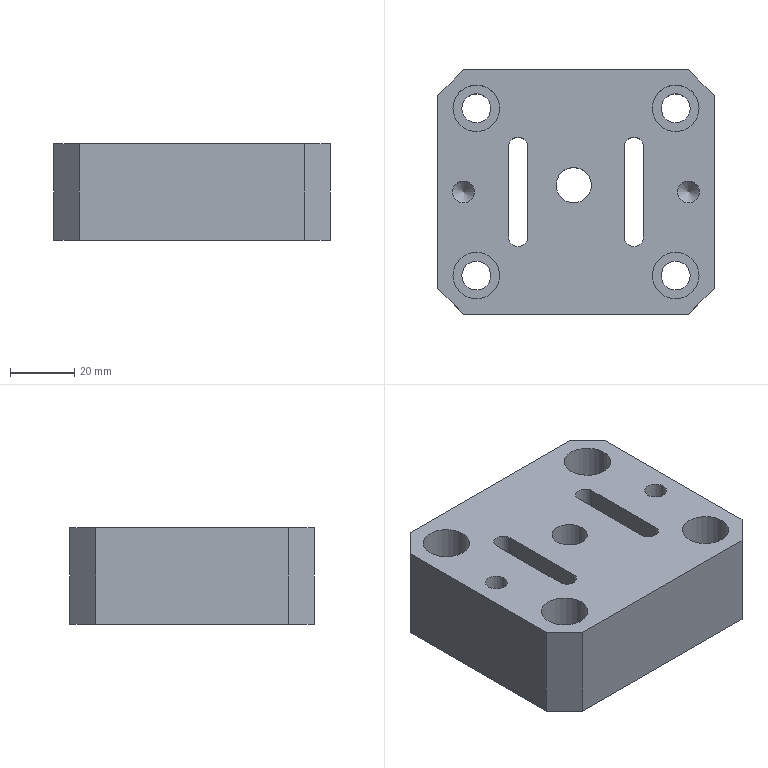Part | NX | features solid 2 | 1 solid | 35 faces | box 86 x 76 x 30 mm | volume 163570 mm3 | plane 18 | cylinder 15 | cone 2 | commonest cylinder face diameters 6 x4 9 x4 14.5 x4 6.8 x2 11 x1
STEP:
#1=CARTESIAN_POINT('',(-104.306,-16.102,-31.5));
#2=VERTEX_POINT('',#1);
#3=CARTESIAN_POINT('',(-110.306,-16.102,-31.5));
#4=VERTEX_POINT('',#3);
#5=CARTESIAN_POINT('',(-107.306,-16.102,-31.5));
#6=DIRECTION('',(0.,0.,-1.));
#7=DIRECTION('',(-1.,0.,0.));
#8=AXIS2_PLACEMENT_3D('',#5,#6,#7);
#9=CIRCLE('',#8,3.);
#10=EDGE_CURVE('',#2,#4,#9,.T.);
#11=ORIENTED_EDGE('',*,*,#10,.F.);
#12=CARTESIAN_POINT('',(-104.306,11.898,-31.5));
#13=VERTEX_POINT('',#12);
#14=CARTESIAN_POINT('',(-104.306,-2.09,-31.5));
#15=DIRECTION('',(0.,-1.,0.));
#16=VECTOR('',#15,1000.);
#17=LINE('',#14,#16);
#18=EDGE_CURVE('',#2,#13,#17,.F.);
#19=ORIENTED_EDGE('',*,*,#18,.T.);
#20=CARTESIAN_POINT('',(-110.306,11.898,-31.5));
#21=VERTEX_POINT('',#20);
#22=CARTESIAN_POINT('',(-107.306,11.898,-31.5));
#23=DIRECTION('',(0.,0.,-1.));
#24=DIRECTION('',(-1.,0.,0.));
#25=AXIS2_PLACEMENT_3D('',#22,#23,#24);
#26=CIRCLE('',#25,3.);
#27=EDGE_CURVE('',#21,#13,#26,.T.);
#28=ORIENTED_EDGE('',*,*,#27,.F.);
#29=CARTESIAN_POINT('',(-110.306,-2.09,-31.5));
#30=DIRECTION('',(0.,1.,0.));
#31=VECTOR('',#30,1000.);
#32=LINE('',#29,#31);
#33=EDGE_CURVE('',#21,#4,#32,.F.);
#34=ORIENTED_EDGE('',*,*,#33,.T.);
#35=EDGE_LOOP('',(#11,#19,#28,#34));
#36=FACE_BOUND('',#35,.T.);
#37=CARTESIAN_POINT('',(-115.803,23.91,-31.5));
#38=VERTEX_POINT('',#37);
#39=CARTESIAN_POINT('',(-120.303,23.91,-31.5));
#40=DIRECTION('',(0.,0.,1.));
#41=DIRECTION('',(1.,0.,0.));
#42=AXIS2_PLACEMENT_3D('',#39,#40,#41);
#43=CIRCLE('',#42,4.5);
#44=EDGE_CURVE('',#38,#38,#43,.T.);
#45=ORIENTED_EDGE('',*,*,#44,.T.);
#46=EDGE_LOOP('',(#45));
#47=FACE_BOUND('',#46,.T.);
#48=CARTESIAN_POINT('',(-53.803,-28.09,-31.5));
#49=VERTEX_POINT('',#48);
#50=CARTESIAN_POINT('',(-58.303,-28.09,-31.5));
#51=DIRECTION('',(0.,0.,1.));
#52=DIRECTION('',(1.,0.,0.));
#53=AXIS2_PLACEMENT_3D('',#50,#51,#52);
#54=CIRCLE('',#53,4.5);
#55=EDGE_CURVE('',#49,#49,#54,.T.);
#56=ORIENTED_EDGE('',*,*,#55,.T.);
#57=EDGE_LOOP('',(#56));
#58=FACE_BOUND('',#57,.T.);
#59=CARTESIAN_POINT('',(-53.803,23.91,-31.5));
#60=VERTEX_POINT('',#59);
#61=CARTESIAN_POINT('',(-58.303,23.91,-31.5));
#62=DIRECTION('',(0.,0.,1.));
#63=DIRECTION('',(1.,0.,0.));
#64=AXIS2_PLACEMENT_3D('',#61,#62,#63);
#65=CIRCLE('',#64,4.5);
#66=EDGE_CURVE('',#60,#60,#65,.T.);
#67=ORIENTED_EDGE('',*,*,#66,.T.);
#68=EDGE_LOOP('',(#67));
#69=FACE_BOUND('',#68,.T.);
#70=CARTESIAN_POINT('',(-115.803,-28.09,-31.5));
#71=VERTEX_POINT('',#70);
#72=CARTESIAN_POINT('',(-120.303,-28.09,-31.5));
#73=DIRECTION('',(0.,0.,1.));
#74=DIRECTION('',(1.,0.,0.));
#75=AXIS2_PLACEMENT_3D('',#72,#73,#74);
#76=CIRCLE('',#75,4.5);
#77=EDGE_CURVE('',#71,#71,#76,.T.);
#78=ORIENTED_EDGE('',*,*,#77,.T.);
#79=EDGE_LOOP('',(#78));
#80=FACE_BOUND('',#79,.T.);
#81=CARTESIAN_POINT('',(-132.303,-32.09,-31.5));
#82=VERTEX_POINT('',#81);
#83=CARTESIAN_POINT('',(-132.303,27.91,-31.5));
#84=VERTEX_POINT('',#83);
#85=CARTESIAN_POINT('',(-132.303,-2.09,-31.5));
#86=DIRECTION('',(0.,1.,0.));
#87=VECTOR('',#86,1000.);
#88=LINE('',#85,#87);
#89=EDGE_CURVE('',#82,#84,#88,.T.);
#90=ORIENTED_EDGE('',*,*,#89,.T.);
#91=CARTESIAN_POINT('',(-124.303,35.91,-31.5));
#92=VERTEX_POINT('',#91);
#93=CARTESIAN_POINT('',(-125.803,34.41,-31.5));
#94=DIRECTION('',(-0.7071,-0.7071,0.));
#95=VECTOR('',#94,1000.);
#96=LINE('',#93,#95);
#97=EDGE_CURVE('',#84,#92,#96,.F.);
#98=ORIENTED_EDGE('',*,*,#97,.T.);
#99=CARTESIAN_POINT('',(-54.303,35.91,-31.5));
#100=VERTEX_POINT('',#99);
#101=CARTESIAN_POINT('',(-89.303,35.91,-31.5));
#102=DIRECTION('',(1.,0.,0.));
#103=VECTOR('',#102,1000.);
#104=LINE('',#101,#103);
#105=EDGE_CURVE('',#92,#100,#104,.T.);
#106=ORIENTED_EDGE('',*,*,#105,.T.);
#107=CARTESIAN_POINT('',(-46.303,27.91,-31.5));
#108=VERTEX_POINT('',#107);
#109=CARTESIAN_POINT('',(-52.803,34.41,-31.5));
#110=DIRECTION('',(-0.7071,0.7071,0.));
#111=VECTOR('',#110,1000.);
#112=LINE('',#109,#111);
#113=EDGE_CURVE('',#100,#108,#112,.F.);
#114=ORIENTED_EDGE('',*,*,#113,.T.);
#115=CARTESIAN_POINT('',(-46.303,-32.09,-31.5));
#116=VERTEX_POINT('',#115);
#117=CARTESIAN_POINT('',(-46.303,-2.09,-31.5));
#118=DIRECTION('',(0.,-1.,0.));
#119=VECTOR('',#118,1000.);
#120=LINE('',#117,#119);
#121=EDGE_CURVE('',#108,#116,#120,.T.);
#122=ORIENTED_EDGE('',*,*,#121,.T.);
#123=CARTESIAN_POINT('',(-54.303,-40.09,-31.5));
#124=VERTEX_POINT('',#123);
#125=CARTESIAN_POINT('',(-52.803,-38.59,-31.5));
#126=DIRECTION('',(0.7071,0.7071,0.));
#127=VECTOR('',#126,1000.);
#128=LINE('',#125,#127);
#129=EDGE_CURVE('',#116,#124,#128,.F.);
#130=ORIENTED_EDGE('',*,*,#129,.T.);
#131=CARTESIAN_POINT('',(-124.303,-40.09,-31.5));
#132=VERTEX_POINT('',#131);
#133=CARTESIAN_POINT('',(-89.303,-40.09,-31.5));
#134=DIRECTION('',(-1.,0.,0.));
#135=VECTOR('',#134,1000.);
#136=LINE('',#133,#135);
#137=EDGE_CURVE('',#124,#132,#136,.T.);
#138=ORIENTED_EDGE('',*,*,#137,.T.);
#139=CARTESIAN_POINT('',(-125.803,-38.59,-31.5));
#140=DIRECTION('',(0.7071,-0.7071,0.));
#141=VECTOR('',#140,1000.);
#142=LINE('',#139,#141);
#143=EDGE_CURVE('',#132,#82,#142,.F.);
#144=ORIENTED_EDGE('',*,*,#143,.T.);
#145=EDGE_LOOP('',(#90,#98,#106,#114,#122,#130,#138,#144));
#146=FACE_BOUND('',#145,.T.);
#147=CARTESIAN_POINT('',(-95.5,0.,-31.5));
#148=VERTEX_POINT('',#147);
#149=CARTESIAN_POINT('',(-90.,0.,-31.5));
#150=DIRECTION('',(0.,0.,-1.));
#151=DIRECTION('',(-1.,0.,0.));
#152=AXIS2_PLACEMENT_3D('',#149,#150,#151);
#153=CIRCLE('',#152,5.5);
#154=EDGE_CURVE('',#148,#148,#153,.T.);
#155=ORIENTED_EDGE('',*,*,#154,.F.);
#156=EDGE_LOOP('',(#155));
#157=FACE_BOUND('',#156,.T.);
#158=CARTESIAN_POINT('',(-74.306,-16.102,-31.5));
#159=VERTEX_POINT('',#158);
#160=CARTESIAN_POINT('',(-68.306,-16.102,-31.5));
#161=VERTEX_POINT('',#160);
#162=CARTESIAN_POINT('',(-71.306,-16.102,-31.5));
#163=DIRECTION('',(0.,0.,-1.));
#164=DIRECTION('',(-1.,0.,0.));
#165=AXIS2_PLACEMENT_3D('',#162,#163,#164);
#166=CIRCLE('',#165,3.);
#167=EDGE_CURVE('',#159,#161,#166,.F.);
#168=ORIENTED_EDGE('',*,*,#167,.T.);
#169=CARTESIAN_POINT('',(-68.306,11.898,-31.5));
#170=VERTEX_POINT('',#169);
#171=CARTESIAN_POINT('',(-68.306,-16.102,-31.5));
#172=DIRECTION('',(0.,1.,0.));
#173=VECTOR('',#172,1000.);
#174=LINE('',#171,#173);
#175=EDGE_CURVE('',#170,#161,#174,.F.);
#176=ORIENTED_EDGE('',*,*,#175,.F.);
#177=CARTESIAN_POINT('',(-74.306,11.898,-31.5));
#178=VERTEX_POINT('',#177);
#179=CARTESIAN_POINT('',(-71.306,11.898,-31.5));
#180=DIRECTION('',(0.,0.,-1.));
#181=DIRECTION('',(-1.,0.,0.));
#182=AXIS2_PLACEMENT_3D('',#179,#180,#181);
#183=CIRCLE('',#182,3.);
#184=EDGE_CURVE('',#170,#178,#183,.F.);
#185=ORIENTED_EDGE('',*,*,#184,.T.);
#186=CARTESIAN_POINT('',(-74.306,-16.102,-31.5));
#187=DIRECTION('',(0.,-1.,0.));
#188=VECTOR('',#187,1000.);
#189=LINE('',#186,#188);
#190=EDGE_CURVE('',#159,#178,#189,.F.);
#191=ORIENTED_EDGE('',*,*,#190,.F.);
#192=EDGE_LOOP('',(#168,#176,#185,#191));
#193=FACE_BOUND('',#192,.T.);
#194=CARTESIAN_POINT('',(-89.303,-2.09,-31.5));
#195=DIRECTION('',(0.,0.,-1.));
#196=DIRECTION('',(1.,0.,0.));
#197=AXIS2_PLACEMENT_3D('',#194,#195,#196);
#198=PLANE('',#197);
#199=ADVANCED_FACE('',(#36,#47,#58,#69,#80,#146,#157,#193),#198,.T.);
#200=CARTESIAN_POINT('',(-74.306,-16.102,-1.5));
#201=VERTEX_POINT('',#200);
#202=CARTESIAN_POINT('',(-68.306,-16.102,-1.5));
#203=VERTEX_POINT('',#202);
#204=CARTESIAN_POINT('',(-71.306,-16.102,-1.5));
#205=DIRECTION('',(0.,0.,1.));
#206=DIRECTION('',(1.,0.,0.));
#207=AXIS2_PLACEMENT_3D('',#204,#205,#206);
#208=CIRCLE('',#207,3.);
#209=EDGE_CURVE('',#201,#203,#208,.T.);
#210=ORIENTED_EDGE('',*,*,#209,.F.);
#211=CARTESIAN_POINT('',(-74.306,11.898,-1.5));
#212=VERTEX_POINT('',#211);
#213=CARTESIAN_POINT('',(-74.306,-2.09,-1.5));
#214=DIRECTION('',(0.,-1.,0.));
#215=VECTOR('',#214,1000.);
#216=LINE('',#213,#215);
#217=EDGE_CURVE('',#212,#201,#216,.T.);
#218=ORIENTED_EDGE('',*,*,#217,.F.);
#219=CARTESIAN_POINT('',(-68.306,11.898,-1.5));
#220=VERTEX_POINT('',#219);
#221=CARTESIAN_POINT('',(-71.306,11.898,-1.5));
#222=DIRECTION('',(0.,0.,1.));
#223=DIRECTION('',(1.,0.,0.));
#224=AXIS2_PLACEMENT_3D('',#221,#222,#223);
#225=CIRCLE('',#224,3.);
#226=EDGE_CURVE('',#220,#212,#225,.T.);
#227=ORIENTED_EDGE('',*,*,#226,.F.);
#228=CARTESIAN_POINT('',(-68.306,-2.09,-1.5));
#229=DIRECTION('',(0.,1.,0.));
#230=VECTOR('',#229,1000.);
#231=LINE('',#228,#230);
#232=EDGE_CURVE('',#203,#220,#231,.T.);
#233=ORIENTED_EDGE('',*,*,#232,.F.);
#234=EDGE_LOOP('',(#210,#218,#227,#233));
#235=FACE_BOUND('',#234,.T.);
#236=CARTESIAN_POINT('',(-110.306,-16.102,-1.5));
#237=VERTEX_POINT('',#236);
#238=CARTESIAN_POINT('',(-104.306,-16.102,-1.5));
#239=VERTEX_POINT('',#238);
#240=CARTESIAN_POINT('',(-107.306,-16.102,-1.5));
#241=DIRECTION('',(0.,0.,1.));
#242=DIRECTION('',(1.,0.,0.));
#243=AXIS2_PLACEMENT_3D('',#240,#241,#242);
#244=CIRCLE('',#243,3.);
#245=EDGE_CURVE('',#237,#239,#244,.T.);
#246=ORIENTED_EDGE('',*,*,#245,.F.);
#247=CARTESIAN_POINT('',(-110.306,11.898,-1.5));
#248=VERTEX_POINT('',#247);
#249=CARTESIAN_POINT('',(-110.306,-2.09,-1.5));
#250=DIRECTION('',(0.,-1.,0.));
#251=VECTOR('',#250,1000.);
#252=LINE('',#249,#251);
#253=EDGE_CURVE('',#248,#237,#252,.T.);
#254=ORIENTED_EDGE('',*,*,#253,.F.);
#255=CARTESIAN_POINT('',(-104.306,11.898,-1.5));
#256=VERTEX_POINT('',#255);
#257=CARTESIAN_POINT('',(-107.306,11.898,-1.5));
#258=DIRECTION('',(0.,0.,1.));
#259=DIRECTION('',(1.,0.,0.));
#260=AXIS2_PLACEMENT_3D('',#257,#258,#259);
#261=CIRCLE('',#260,3.);
#262=EDGE_CURVE('',#256,#248,#261,.T.);
#263=ORIENTED_EDGE('',*,*,#262,.F.);
#264=CARTESIAN_POINT('',(-104.306,-2.09,-1.5));
#265=DIRECTION('',(0.,1.,0.));
#266=VECTOR('',#265,1000.);
#267=LINE('',#264,#266);
#268=EDGE_CURVE('',#239,#256,#267,.T.);
#269=ORIENTED_EDGE('',*,*,#268,.F.);
#270=EDGE_LOOP('',(#246,#254,#263,#269));
#271=FACE_BOUND('',#270,.T.);
#272=CARTESIAN_POINT('',(-57.703,-2.09,-1.5));
#273=VERTEX_POINT('',#272);
#274=CARTESIAN_POINT('',(-54.303,-2.09,-1.5));
#275=DIRECTION('',(0.,0.,1.));
#276=DIRECTION('',(-1.,0.,0.));
#277=AXIS2_PLACEMENT_3D('',#274,#275,#276);
#278=CIRCLE('',#277,3.4);
#279=EDGE_CURVE('',#273,#273,#278,.T.);
#280=ORIENTED_EDGE('',*,*,#279,.F.);
#281=EDGE_LOOP('',(#280));
#282=FACE_BOUND('',#281,.T.);
#283=CARTESIAN_POINT('',(-120.903,-2.09,-1.5));
#284=VERTEX_POINT('',#283);
#285=CARTESIAN_POINT('',(-124.303,-2.09,-1.5));
#286=DIRECTION('',(0.,0.,-1.));
#287=DIRECTION('',(1.,0.,0.));
#288=AXIS2_PLACEMENT_3D('',#285,#286,#287);
#289=CIRCLE('',#288,3.4);
#290=EDGE_CURVE('',#284,#284,#289,.T.);
#291=ORIENTED_EDGE('',*,*,#290,.T.);
#292=EDGE_LOOP('',(#291));
#293=FACE_BOUND('',#292,.T.);
#294=CARTESIAN_POINT('',(-51.053,-28.09,-1.5));
#295=VERTEX_POINT('',#294);
#296=CARTESIAN_POINT('',(-58.303,-28.09,-1.5));
#297=DIRECTION('',(0.,0.,1.));
#298=DIRECTION('',(1.,0.,0.));
#299=AXIS2_PLACEMENT_3D('',#296,#297,#298);
#300=CIRCLE('',#299,7.25);
#301=EDGE_CURVE('',#295,#295,#300,.T.);
#302=ORIENTED_EDGE('',*,*,#301,.F.);
#303=EDGE_LOOP('',(#302));
#304=FACE_BOUND('',#303,.T.);
#305=CARTESIAN_POINT('',(-113.053,-28.09,-1.5));
#306=VERTEX_POINT('',#305);
#307=CARTESIAN_POINT('',(-120.303,-28.09,-1.5));
#308=DIRECTION('',(0.,0.,1.));
#309=DIRECTION('',(1.,0.,0.));
#310=AXIS2_PLACEMENT_3D('',#307,#308,#309);
#311=CIRCLE('',#310,7.25);
#312=EDGE_CURVE('',#306,#306,#311,.T.);
#313=ORIENTED_EDGE('',*,*,#312,.F.);
#314=EDGE_LOOP('',(#313));
#315=FACE_BOUND('',#314,.T.);
#316=CARTESIAN_POINT('',(-54.303,35.91,-1.5));
#317=VERTEX_POINT('',#316);
#318=CARTESIAN_POINT('',(-124.303,35.91,-1.5));
#319=VERTEX_POINT('',#318);
#320=CARTESIAN_POINT('',(-89.303,35.91,-1.5));
#321=DIRECTION('',(-1.,0.,0.));
#322=VECTOR('',#321,1000.);
#323=LINE('',#320,#322);
#324=EDGE_CURVE('',#317,#319,#323,.T.);
#325=ORIENTED_EDGE('',*,*,#324,.T.);
#326=CARTESIAN_POINT('',(-132.303,27.91,-1.5));
#327=VERTEX_POINT('',#326);
#328=CARTESIAN_POINT('',(-125.803,34.41,-1.5));
#329=DIRECTION('',(0.7071,0.7071,0.));
#330=VECTOR('',#329,1000.);
#331=LINE('',#328,#330);
#332=EDGE_CURVE('',#319,#327,#331,.F.);
#333=ORIENTED_EDGE('',*,*,#332,.T.);
#334=CARTESIAN_POINT('',(-132.303,-32.09,-1.5));
#335=VERTEX_POINT('',#334);
#336=CARTESIAN_POINT('',(-132.303,-2.09,-1.5));
#337=DIRECTION('',(0.,-1.,0.));
#338=VECTOR('',#337,1000.);
#339=LINE('',#336,#338);
#340=EDGE_CURVE('',#327,#335,#339,.T.);
#341=ORIENTED_EDGE('',*,*,#340,.T.);
#342=CARTESIAN_POINT('',(-124.303,-40.09,-1.5));
#343=VERTEX_POINT('',#342);
#344=CARTESIAN_POINT('',(-125.803,-38.59,-1.5));
#345=DIRECTION('',(-0.7071,0.7071,0.));
#346=VECTOR('',#345,1000.);
#347=LINE('',#344,#346);
#348=EDGE_CURVE('',#335,#343,#347,.F.);
#349=ORIENTED_EDGE('',*,*,#348,.T.);
#350=CARTESIAN_POINT('',(-54.303,-40.09,-1.5));
#351=VERTEX_POINT('',#350);
#352=CARTESIAN_POINT('',(-89.303,-40.09,-1.5));
#353=DIRECTION('',(1.,0.,0.));
#354=VECTOR('',#353,1000.);
#355=LINE('',#352,#354);
#356=EDGE_CURVE('',#343,#351,#355,.T.);
#357=ORIENTED_EDGE('',*,*,#356,.T.);
#358=CARTESIAN_POINT('',(-46.303,-32.09,-1.5));
#359=VERTEX_POINT('',#358);
#360=CARTESIAN_POINT('',(-52.803,-38.59,-1.5));
#361=DIRECTION('',(-0.7071,-0.7071,0.));
#362=VECTOR('',#361,1000.);
#363=LINE('',#360,#362);
#364=EDGE_CURVE('',#351,#359,#363,.F.);
#365=ORIENTED_EDGE('',*,*,#364,.T.);
#366=CARTESIAN_POINT('',(-46.303,27.91,-1.5));
#367=VERTEX_POINT('',#366);
#368=CARTESIAN_POINT('',(-46.303,-2.09,-1.5));
#369=DIRECTION('',(0.,1.,0.));
#370=VECTOR('',#369,1000.);
#371=LINE('',#368,#370);
#372=EDGE_CURVE('',#359,#367,#371,.T.);
#373=ORIENTED_EDGE('',*,*,#372,.T.);
#374=CARTESIAN_POINT('',(-52.803,34.41,-1.5));
#375=DIRECTION('',(0.7071,-0.7071,0.));
#376=VECTOR('',#375,1000.);
#377=LINE('',#374,#376);
#378=EDGE_CURVE('',#367,#317,#377,.F.);
#379=ORIENTED_EDGE('',*,*,#378,.T.);
#380=EDGE_LOOP('',(#325,#333,#341,#349,#357,#365,#373,#379));
#381=FACE_BOUND('',#380,.T.);
#382=CARTESIAN_POINT('',(-51.053,23.91,-1.5));
#383=VERTEX_POINT('',#382);
#384=CARTESIAN_POINT('',(-58.303,23.91,-1.5));
#385=DIRECTION('',(0.,0.,1.));
#386=DIRECTION('',(1.,0.,0.));
#387=AXIS2_PLACEMENT_3D('',#384,#385,#386);
#388=CIRCLE('',#387,7.25);
#389=EDGE_CURVE('',#383,#383,#388,.T.);
#390=ORIENTED_EDGE('',*,*,#389,.F.);
#391=EDGE_LOOP('',(#390));
#392=FACE_BOUND('',#391,.T.);
#393=CARTESIAN_POINT('',(-113.053,23.91,-1.5));
#394=VERTEX_POINT('',#393);
#395=CARTESIAN_POINT('',(-120.303,23.91,-1.5));
#396=DIRECTION('',(0.,0.,1.));
#397=DIRECTION('',(1.,0.,0.));
#398=AXIS2_PLACEMENT_3D('',#395,#396,#397);
#399=CIRCLE('',#398,7.25);
#400=EDGE_CURVE('',#394,#394,#399,.T.);
#401=ORIENTED_EDGE('',*,*,#400,.F.);
#402=EDGE_LOOP('',(#401));
#403=FACE_BOUND('',#402,.T.);
#404=CARTESIAN_POINT('',(-84.5,0.,-1.5));
#405=VERTEX_POINT('',#404);
#406=CARTESIAN_POINT('',(-90.,0.,-1.5));
#407=DIRECTION('',(0.,0.,1.));
#408=DIRECTION('',(1.,0.,0.));
#409=AXIS2_PLACEMENT_3D('',#406,#407,#408);
#410=CIRCLE('',#409,5.5);
#411=EDGE_CURVE('',#405,#405,#410,.T.);
#412=ORIENTED_EDGE('',*,*,#411,.F.);
#413=EDGE_LOOP('',(#412));
#414=FACE_BOUND('',#413,.T.);
#415=CARTESIAN_POINT('',(-89.303,-2.09,-1.5));
#416=DIRECTION('',(0.,0.,1.));
#417=DIRECTION('',(-1.,0.,0.));
#418=AXIS2_PLACEMENT_3D('',#415,#416,#417);
#419=PLANE('',#418);
#420=ADVANCED_FACE('',(#235,#271,#282,#293,#304,#315,#381,#392,#403,#414),#419,.T.);
#421=ORIENTED_EDGE('',*,*,#356,.F.);
#422=CARTESIAN_POINT('',(-124.303,-40.09,-1.5));
#423=DIRECTION('',(0.,0.,-1.));
#424=VECTOR('',#423,1000.);
#425=LINE('',#422,#424);
#426=EDGE_CURVE('',#343,#132,#425,.T.);
#427=ORIENTED_EDGE('',*,*,#426,.T.);
#428=ORIENTED_EDGE('',*,*,#137,.F.);
#429=CARTESIAN_POINT('',(-54.303,-40.09,-1.5));
#430=DIRECTION('',(0.,0.,1.));
#431=VECTOR('',#430,1000.);
#432=LINE('',#429,#431);
#433=EDGE_CURVE('',#124,#351,#432,.T.);
#434=ORIENTED_EDGE('',*,*,#433,.T.);
#435=EDGE_LOOP('',(#421,#427,#428,#434));
#436=FACE_BOUND('',#435,.T.);
#437=CARTESIAN_POINT('',(-89.303,-40.09,-1.5));
#438=DIRECTION('',(0.,-1.,0.));
#439=DIRECTION('',(0.,0.,1.));
#440=AXIS2_PLACEMENT_3D('',#437,#438,#439);
#441=PLANE('',#440);
#442=ADVANCED_FACE('',(#436),#441,.T.);
#443=ORIENTED_EDGE('',*,*,#340,.F.);
#444=CARTESIAN_POINT('',(-132.303,27.91,-1.5));
#445=DIRECTION('',(0.,0.,-1.));
#446=VECTOR('',#445,1000.);
#447=LINE('',#444,#446);
#448=EDGE_CURVE('',#327,#84,#447,.T.);
#449=ORIENTED_EDGE('',*,*,#448,.T.);
#450=ORIENTED_EDGE('',*,*,#89,.F.);
#451=CARTESIAN_POINT('',(-132.303,-32.09,-1.5));
#452=DIRECTION('',(0.,0.,1.));
#453=VECTOR('',#452,1000.);
#454=LINE('',#451,#453);
#455=EDGE_CURVE('',#82,#335,#454,.T.);
#456=ORIENTED_EDGE('',*,*,#455,.T.);
#457=EDGE_LOOP('',(#443,#449,#450,#456));
#458=FACE_BOUND('',#457,.T.);
#459=CARTESIAN_POINT('',(-132.303,-2.09,-1.5));
#460=DIRECTION('',(-1.,0.,0.));
#461=DIRECTION('',(0.,0.,-1.));
#462=AXIS2_PLACEMENT_3D('',#459,#460,#461);
#463=PLANE('',#462);
#464=ADVANCED_FACE('',(#458),#463,.T.);
#465=ORIENTED_EDGE('',*,*,#105,.F.);
#466=CARTESIAN_POINT('',(-124.303,35.91,-1.5));
#467=DIRECTION('',(0.,0.,1.));
#468=VECTOR('',#467,1000.);
#469=LINE('',#466,#468);
#470=EDGE_CURVE('',#92,#319,#469,.T.);
#471=ORIENTED_EDGE('',*,*,#470,.T.);
#472=ORIENTED_EDGE('',*,*,#324,.F.);
#473=CARTESIAN_POINT('',(-54.303,35.91,-1.5));
#474=DIRECTION('',(0.,0.,-1.));
#475=VECTOR('',#474,1000.);
#476=LINE('',#473,#475);
#477=EDGE_CURVE('',#317,#100,#476,.T.);
#478=ORIENTED_EDGE('',*,*,#477,.T.);
#479=EDGE_LOOP('',(#465,#471,#472,#478));
#480=FACE_BOUND('',#479,.T.);
#481=CARTESIAN_POINT('',(-89.303,35.91,-1.5));
#482=DIRECTION('',(0.,1.,0.));
#483=DIRECTION('',(0.,0.,-1.));
#484=AXIS2_PLACEMENT_3D('',#481,#482,#483);
#485=PLANE('',#484);
#486=ADVANCED_FACE('',(#480),#485,.T.);
#487=ORIENTED_EDGE('',*,*,#372,.F.);
#488=CARTESIAN_POINT('',(-46.303,-32.09,-1.5));
#489=DIRECTION('',(0.,0.,-1.));
#490=VECTOR('',#489,1000.);
#491=LINE('',#488,#490);
#492=EDGE_CURVE('',#359,#116,#491,.T.);
#493=ORIENTED_EDGE('',*,*,#492,.T.);
#494=ORIENTED_EDGE('',*,*,#121,.F.);
#495=CARTESIAN_POINT('',(-46.303,27.91,-1.5));
#496=DIRECTION('',(0.,0.,1.));
#497=VECTOR('',#496,1000.);
#498=LINE('',#495,#497);
#499=EDGE_CURVE('',#108,#367,#498,.T.);
#500=ORIENTED_EDGE('',*,*,#499,.T.);
#501=EDGE_LOOP('',(#487,#493,#494,#500));
#502=FACE_BOUND('',#501,.T.);
#503=CARTESIAN_POINT('',(-46.303,-2.09,-1.5));
#504=DIRECTION('',(1.,0.,0.));
#505=DIRECTION('',(0.,0.,1.));
#506=AXIS2_PLACEMENT_3D('',#503,#504,#505);
#507=PLANE('',#506);
#508=ADVANCED_FACE('',(#502),#507,.T.);
#509=ORIENTED_EDGE('',*,*,#77,.F.);
#510=EDGE_LOOP('',(#509));
#511=FACE_BOUND('',#510,.T.);
#512=CARTESIAN_POINT('',(-115.803,-28.09,-12.5));
#513=VERTEX_POINT('',#512);
#514=CARTESIAN_POINT('',(-120.303,-28.09,-12.5));
#515=DIRECTION('',(0.,0.,1.));
#516=DIRECTION('',(1.,0.,0.));
#517=AXIS2_PLACEMENT_3D('',#514,#515,#516);
#518=CIRCLE('',#517,4.5);
#519=EDGE_CURVE('',#513,#513,#518,.T.);
#520=ORIENTED_EDGE('',*,*,#519,.T.);
#521=EDGE_LOOP('',(#520));
#522=FACE_BOUND('',#521,.T.);
#523=CARTESIAN_POINT('',(-120.303,-28.09,1.5));
#524=DIRECTION('',(0.,0.,-1.));
#525=DIRECTION('',(1.,0.,0.));
#526=AXIS2_PLACEMENT_3D('',#523,#524,#525);
#527=CYLINDRICAL_SURFACE('',#526,4.5);
#528=ADVANCED_FACE('',(#511,#522),#527,.F.);
#529=ORIENTED_EDGE('',*,*,#519,.F.);
#530=EDGE_LOOP('',(#529));
#531=FACE_BOUND('',#530,.T.);
#532=CARTESIAN_POINT('',(-113.053,-28.09,-12.5));
#533=VERTEX_POINT('',#532);
#534=CARTESIAN_POINT('',(-120.303,-28.09,-12.5));
#535=DIRECTION('',(0.,0.,-1.));
#536=DIRECTION('',(1.,0.,0.));
#537=AXIS2_PLACEMENT_3D('',#534,#535,#536);
#538=CIRCLE('',#537,7.25);
#539=EDGE_CURVE('',#533,#533,#538,.F.);
#540=ORIENTED_EDGE('',*,*,#539,.T.);
#541=EDGE_LOOP('',(#540));
#542=FACE_BOUND('',#541,.T.);
#543=CARTESIAN_POINT('',(-120.303,-28.09,-12.5));
#544=DIRECTION('',(0.,0.,-1.));
#545=DIRECTION('',(1.,0.,0.));
#546=AXIS2_PLACEMENT_3D('',#543,#544,#545);
#547=PLANE('',#546);
#548=ADVANCED_FACE('',(#531,#542),#547,.F.);
#549=ORIENTED_EDGE('',*,*,#539,.F.);
#550=EDGE_LOOP('',(#549));
#551=FACE_BOUND('',#550,.T.);
#552=ORIENTED_EDGE('',*,*,#312,.T.);
#553=EDGE_LOOP('',(#552));
#554=FACE_BOUND('',#553,.T.);
#555=CARTESIAN_POINT('',(-120.303,-28.09,-1.5));
#556=DIRECTION('',(0.,0.,-1.));
#557=DIRECTION('',(1.,0.,0.));
#558=AXIS2_PLACEMENT_3D('',#555,#556,#557);
#559=CYLINDRICAL_SURFACE('',#558,7.25);
#560=ADVANCED_FACE('',(#551,#554),#559,.F.);
#561=ORIENTED_EDGE('',*,*,#66,.F.);
#562=EDGE_LOOP('',(#561));
#563=FACE_BOUND('',#562,.T.);
#564=CARTESIAN_POINT('',(-53.803,23.91,-12.5));
#565=VERTEX_POINT('',#564);
#566=CARTESIAN_POINT('',(-58.303,23.91,-12.5));
#567=DIRECTION('',(0.,0.,1.));
#568=DIRECTION('',(1.,0.,0.));
#569=AXIS2_PLACEMENT_3D('',#566,#567,#568);
#570=CIRCLE('',#569,4.5);
#571=EDGE_CURVE('',#565,#565,#570,.T.);
#572=ORIENTED_EDGE('',*,*,#571,.T.);
#573=EDGE_LOOP('',(#572));
#574=FACE_BOUND('',#573,.T.);
#575=CARTESIAN_POINT('',(-58.303,23.91,1.5));
#576=DIRECTION('',(0.,0.,-1.));
#577=DIRECTION('',(1.,0.,0.));
#578=AXIS2_PLACEMENT_3D('',#575,#576,#577);
#579=CYLINDRICAL_SURFACE('',#578,4.5);
#580=ADVANCED_FACE('',(#563,#574),#579,.F.);
#581=ORIENTED_EDGE('',*,*,#571,.F.);
#582=EDGE_LOOP('',(#581));
#583=FACE_BOUND('',#582,.T.);
#584=CARTESIAN_POINT('',(-51.053,23.91,-12.5));
#585=VERTEX_POINT('',#584);
#586=CARTESIAN_POINT('',(-58.303,23.91,-12.5));
#587=DIRECTION('',(0.,0.,-1.));
#588=DIRECTION('',(1.,0.,0.));
#589=AXIS2_PLACEMENT_3D('',#586,#587,#588);
#590=CIRCLE('',#589,7.25);
#591=EDGE_CURVE('',#585,#585,#590,.F.);
#592=ORIENTED_EDGE('',*,*,#591,.T.);
#593=EDGE_LOOP('',(#592));
#594=FACE_BOUND('',#593,.T.);
#595=CARTESIAN_POINT('',(-58.303,23.91,-12.5));
#596=DIRECTION('',(0.,0.,-1.));
#597=DIRECTION('',(1.,0.,0.));
#598=AXIS2_PLACEMENT_3D('',#595,#596,#597);
#599=PLANE('',#598);
#600=ADVANCED_FACE('',(#583,#594),#599,.F.);
#601=ORIENTED_EDGE('',*,*,#591,.F.);
#602=EDGE_LOOP('',(#601));
#603=FACE_BOUND('',#602,.T.);
#604=ORIENTED_EDGE('',*,*,#389,.T.);
#605=EDGE_LOOP('',(#604));
#606=FACE_BOUND('',#605,.T.);
#607=CARTESIAN_POINT('',(-58.303,23.91,-1.5));
#608=DIRECTION('',(0.,0.,-1.));
#609=DIRECTION('',(1.,0.,0.));
#610=AXIS2_PLACEMENT_3D('',#607,#608,#609);
#611=CYLINDRICAL_SURFACE('',#610,7.25);
#612=ADVANCED_FACE('',(#603,#606),#611,.F.);
#613=ORIENTED_EDGE('',*,*,#55,.F.);
#614=EDGE_LOOP('',(#613));
#615=FACE_BOUND('',#614,.T.);
#616=CARTESIAN_POINT('',(-53.803,-28.09,-12.5));
#617=VERTEX_POINT('',#616);
#618=CARTESIAN_POINT('',(-58.303,-28.09,-12.5));
#619=DIRECTION('',(0.,0.,1.));
#620=DIRECTION('',(1.,0.,0.));
#621=AXIS2_PLACEMENT_3D('',#618,#619,#620);
#622=CIRCLE('',#621,4.5);
#623=EDGE_CURVE('',#617,#617,#622,.T.);
#624=ORIENTED_EDGE('',*,*,#623,.T.);
#625=EDGE_LOOP('',(#624));
#626=FACE_BOUND('',#625,.T.);
#627=CARTESIAN_POINT('',(-58.303,-28.09,1.5));
#628=DIRECTION('',(0.,0.,-1.));
#629=DIRECTION('',(1.,0.,0.));
#630=AXIS2_PLACEMENT_3D('',#627,#628,#629);
#631=CYLINDRICAL_SURFACE('',#630,4.5);
#632=ADVANCED_FACE('',(#615,#626),#631,.F.);
#633=ORIENTED_EDGE('',*,*,#623,.F.);
#634=EDGE_LOOP('',(#633));
#635=FACE_BOUND('',#634,.T.);
#636=CARTESIAN_POINT('',(-51.053,-28.09,-12.5));
#637=VERTEX_POINT('',#636);
#638=CARTESIAN_POINT('',(-58.303,-28.09,-12.5));
#639=DIRECTION('',(0.,0.,-1.));
#640=DIRECTION('',(1.,0.,0.));
#641=AXIS2_PLACEMENT_3D('',#638,#639,#640);
#642=CIRCLE('',#641,7.25);
#643=EDGE_CURVE('',#637,#637,#642,.F.);
#644=ORIENTED_EDGE('',*,*,#643,.T.);
#645=EDGE_LOOP('',(#644));
#646=FACE_BOUND('',#645,.T.);
#647=CARTESIAN_POINT('',(-58.303,-28.09,-12.5));
#648=DIRECTION('',(0.,0.,-1.));
#649=DIRECTION('',(1.,0.,0.));
#650=AXIS2_PLACEMENT_3D('',#647,#648,#649);
#651=PLANE('',#650);
#652=ADVANCED_FACE('',(#635,#646),#651,.F.);
#653=ORIENTED_EDGE('',*,*,#643,.F.);
#654=EDGE_LOOP('',(#653));
#655=FACE_BOUND('',#654,.T.);
#656=ORIENTED_EDGE('',*,*,#301,.T.);
#657=EDGE_LOOP('',(#656));
#658=FACE_BOUND('',#657,.T.);
#659=CARTESIAN_POINT('',(-58.303,-28.09,-1.5));
#660=DIRECTION('',(0.,0.,-1.));
#661=DIRECTION('',(1.,0.,0.));
#662=AXIS2_PLACEMENT_3D('',#659,#660,#661);
#663=CYLINDRICAL_SURFACE('',#662,7.25);
#664=ADVANCED_FACE('',(#655,#658),#663,.F.);
#665=ORIENTED_EDGE('',*,*,#44,.F.);
#666=EDGE_LOOP('',(#665));
#667=FACE_BOUND('',#666,.T.);
#668=CARTESIAN_POINT('',(-115.803,23.91,-12.5));
#669=VERTEX_POINT('',#668);
#670=CARTESIAN_POINT('',(-120.303,23.91,-12.5));
#671=DIRECTION('',(0.,0.,1.));
#672=DIRECTION('',(1.,0.,0.));
#673=AXIS2_PLACEMENT_3D('',#670,#671,#672);
#674=CIRCLE('',#673,4.5);
#675=EDGE_CURVE('',#669,#669,#674,.T.);
#676=ORIENTED_EDGE('',*,*,#675,.T.);
#677=EDGE_LOOP('',(#676));
#678=FACE_BOUND('',#677,.T.);
#679=CARTESIAN_POINT('',(-120.303,23.91,1.5));
#680=DIRECTION('',(0.,0.,-1.));
#681=DIRECTION('',(1.,0.,0.));
#682=AXIS2_PLACEMENT_3D('',#679,#680,#681);
#683=CYLINDRICAL_SURFACE('',#682,4.5);
#684=ADVANCED_FACE('',(#667,#678),#683,.F.);
#685=ORIENTED_EDGE('',*,*,#675,.F.);
#686=EDGE_LOOP('',(#685));
#687=FACE_BOUND('',#686,.T.);
#688=CARTESIAN_POINT('',(-113.053,23.91,-12.5));
#689=VERTEX_POINT('',#688);
#690=CARTESIAN_POINT('',(-120.303,23.91,-12.5));
#691=DIRECTION('',(0.,0.,-1.));
#692=DIRECTION('',(1.,0.,0.));
#693=AXIS2_PLACEMENT_3D('',#690,#691,#692);
#694=CIRCLE('',#693,7.25);
#695=EDGE_CURVE('',#689,#689,#694,.F.);
#696=ORIENTED_EDGE('',*,*,#695,.T.);
#697=EDGE_LOOP('',(#696));
#698=FACE_BOUND('',#697,.T.);
#699=CARTESIAN_POINT('',(-120.303,23.91,-12.5));
#700=DIRECTION('',(0.,0.,-1.));
#701=DIRECTION('',(1.,0.,0.));
#702=AXIS2_PLACEMENT_3D('',#699,#700,#701);
#703=PLANE('',#702);
#704=ADVANCED_FACE('',(#687,#698),#703,.F.);
#705=ORIENTED_EDGE('',*,*,#695,.F.);
#706=EDGE_LOOP('',(#705));
#707=FACE_BOUND('',#706,.T.);
#708=ORIENTED_EDGE('',*,*,#400,.T.);
#709=EDGE_LOOP('',(#708));
#710=FACE_BOUND('',#709,.T.);
#711=CARTESIAN_POINT('',(-120.303,23.91,-1.5));
#712=DIRECTION('',(0.,0.,-1.));
#713=DIRECTION('',(1.,0.,0.));
#714=AXIS2_PLACEMENT_3D('',#711,#712,#713);
#715=CYLINDRICAL_SURFACE('',#714,7.25);
#716=ADVANCED_FACE('',(#707,#710),#715,.F.);
#717=ORIENTED_EDGE('',*,*,#332,.F.);
#718=ORIENTED_EDGE('',*,*,#470,.F.);
#719=ORIENTED_EDGE('',*,*,#97,.F.);
#720=ORIENTED_EDGE('',*,*,#448,.F.);
#721=EDGE_LOOP('',(#717,#718,#719,#720));
#722=FACE_BOUND('',#721,.T.);
#723=CARTESIAN_POINT('',(-132.303,27.91,-1.5));
#724=DIRECTION('',(0.7071,-0.7071,0.));
#725=DIRECTION('',(0.,0.,-1.));
#726=AXIS2_PLACEMENT_3D('',#723,#724,#725);
#727=PLANE('',#726);
#728=ADVANCED_FACE('',(#722),#727,.F.);
#729=ORIENTED_EDGE('',*,*,#348,.F.);
#730=ORIENTED_EDGE('',*,*,#455,.F.);
#731=ORIENTED_EDGE('',*,*,#143,.F.);
#732=ORIENTED_EDGE('',*,*,#426,.F.);
#733=EDGE_LOOP('',(#729,#730,#731,#732));
#734=FACE_BOUND('',#733,.T.);
#735=CARTESIAN_POINT('',(-124.303,-40.09,-1.5));
#736=DIRECTION('',(0.7071,0.7071,0.));
#737=DIRECTION('',(0.,0.,-1.));
#738=AXIS2_PLACEMENT_3D('',#735,#736,#737);
#739=PLANE('',#738);
#740=ADVANCED_FACE('',(#734),#739,.F.);
#741=ORIENTED_EDGE('',*,*,#364,.F.);
#742=ORIENTED_EDGE('',*,*,#433,.F.);
#743=ORIENTED_EDGE('',*,*,#129,.F.);
#744=ORIENTED_EDGE('',*,*,#492,.F.);
#745=EDGE_LOOP('',(#741,#742,#743,#744));
#746=FACE_BOUND('',#745,.T.);
#747=CARTESIAN_POINT('',(-46.303,-32.09,-1.5));
#748=DIRECTION('',(-0.7071,0.7071,0.));
#749=DIRECTION('',(0.,0.,-1.));
#750=AXIS2_PLACEMENT_3D('',#747,#748,#749);
#751=PLANE('',#750);
#752=ADVANCED_FACE('',(#746),#751,.F.);
#753=ORIENTED_EDGE('',*,*,#378,.F.);
#754=ORIENTED_EDGE('',*,*,#499,.F.);
#755=ORIENTED_EDGE('',*,*,#113,.F.);
#756=ORIENTED_EDGE('',*,*,#477,.F.);
#757=EDGE_LOOP('',(#753,#754,#755,#756));
#758=FACE_BOUND('',#757,.T.);
#759=CARTESIAN_POINT('',(-54.303,35.91,-1.5));
#760=DIRECTION('',(-0.7071,-0.7071,0.));
#761=DIRECTION('',(0.,0.,-1.));
#762=AXIS2_PLACEMENT_3D('',#759,#760,#761);
#763=PLANE('',#762);
#764=ADVANCED_FACE('',(#758),#763,.F.);
#765=ORIENTED_EDGE('',*,*,#411,.T.);
#766=EDGE_LOOP('',(#765));
#767=FACE_BOUND('',#766,.T.);
#768=ORIENTED_EDGE('',*,*,#154,.T.);
#769=EDGE_LOOP('',(#768));
#770=FACE_BOUND('',#769,.T.);
#771=CARTESIAN_POINT('',(-90.,0.,-61.501));
#772=DIRECTION('',(0.,0.,1.));
#773=DIRECTION('',(1.,0.,0.));
#774=AXIS2_PLACEMENT_3D('',#771,#772,#773);
#775=CYLINDRICAL_SURFACE('',#774,5.5);
#776=ADVANCED_FACE('',(#767,#770),#775,.F.);
#777=CARTESIAN_POINT('',(-127.703,-2.09,-27.1));
#778=VERTEX_POINT('',#777);
#779=CARTESIAN_POINT('',(-124.303,-2.09,-27.1));
#780=DIRECTION('',(0.,0.,-1.));
#781=DIRECTION('',(-1.,0.,0.));
#782=AXIS2_PLACEMENT_3D('',#779,#780,#781);
#783=CIRCLE('',#782,3.4);
#784=EDGE_CURVE('',#778,#778,#783,.T.);
#785=ORIENTED_EDGE('',*,*,#784,.T.);
#786=EDGE_LOOP('',(#785));
#787=FACE_BOUND('',#786,.T.);
#788=ORIENTED_EDGE('',*,*,#290,.F.);
#789=EDGE_LOOP('',(#788));
#790=FACE_BOUND('',#789,.T.);
#791=CARTESIAN_POINT('',(-124.303,-2.09,-1.5));
#792=DIRECTION('',(0.,0.,-1.));
#793=DIRECTION('',(1.,0.,0.));
#794=AXIS2_PLACEMENT_3D('',#791,#792,#793);
#795=CYLINDRICAL_SURFACE('',#794,3.4);
#796=ADVANCED_FACE('',(#787,#790),#795,.F.);
#797=CARTESIAN_POINT('',(-124.303,-2.09,-30.5));
#798=VERTEX_POINT('',#797);
#799=VERTEX_LOOP('',#798);
#800=FACE_BOUND('',#799,.T.);
#801=ORIENTED_EDGE('',*,*,#784,.F.);
#802=EDGE_LOOP('',(#801));
#803=FACE_BOUND('',#802,.T.);
#804=CARTESIAN_POINT('',(-124.303,-2.09,-27.1));
#805=DIRECTION('',(0.,0.,1.));
#806=DIRECTION('',(1.,0.,0.));
#807=AXIS2_PLACEMENT_3D('',#804,#805,#806);
#808=CONICAL_SURFACE('',#807,3.4,0.7854);
#809=ADVANCED_FACE('',(#800,#803),#808,.F.);
#810=CARTESIAN_POINT('',(-50.903,-2.09,-27.1));
#811=VERTEX_POINT('',#810);
#812=CARTESIAN_POINT('',(-54.303,-2.09,-27.1));
#813=DIRECTION('',(0.,0.,1.));
#814=DIRECTION('',(1.,0.,0.));
#815=AXIS2_PLACEMENT_3D('',#812,#813,#814);
#816=CIRCLE('',#815,3.4);
#817=EDGE_CURVE('',#811,#811,#816,.T.);
#818=ORIENTED_EDGE('',*,*,#817,.F.);
#819=EDGE_LOOP('',(#818));
#820=FACE_BOUND('',#819,.T.);
#821=ORIENTED_EDGE('',*,*,#279,.T.);
#822=EDGE_LOOP('',(#821));
#823=FACE_BOUND('',#822,.T.);
#824=CARTESIAN_POINT('',(-54.303,-2.09,-1.5));
#825=DIRECTION('',(0.,0.,-1.));
#826=DIRECTION('',(-1.,0.,0.));
#827=AXIS2_PLACEMENT_3D('',#824,#825,#826);
#828=CYLINDRICAL_SURFACE('',#827,3.4);
#829=ADVANCED_FACE('',(#820,#823),#828,.F.);
#830=CARTESIAN_POINT('',(-54.303,-2.09,-30.5));
#831=VERTEX_POINT('',#830);
#832=VERTEX_LOOP('',#831);
#833=FACE_BOUND('',#832,.T.);
#834=ORIENTED_EDGE('',*,*,#817,.T.);
#835=EDGE_LOOP('',(#834));
#836=FACE_BOUND('',#835,.T.);
#837=CARTESIAN_POINT('',(-54.303,-2.09,-27.1));
#838=DIRECTION('',(0.,0.,1.));
#839=DIRECTION('',(-1.,0.,0.));
#840=AXIS2_PLACEMENT_3D('',#837,#838,#839);
#841=CONICAL_SURFACE('',#840,3.4,0.7854);
#842=ADVANCED_FACE('',(#833,#836),#841,.F.);
#843=ORIENTED_EDGE('',*,*,#253,.T.);
#844=CARTESIAN_POINT('',(-110.306,-16.102,-5.5));
#845=DIRECTION('',(0.,0.,1.));
#846=VECTOR('',#845,1000.);
#847=LINE('',#844,#846);
#848=EDGE_CURVE('',#4,#237,#847,.T.);
#849=ORIENTED_EDGE('',*,*,#848,.F.);
#850=ORIENTED_EDGE('',*,*,#33,.F.);
#851=CARTESIAN_POINT('',(-110.306,11.898,-5.5));
#852=DIRECTION('',(0.,0.,1.));
#853=VECTOR('',#852,1000.);
#854=LINE('',#851,#853);
#855=EDGE_CURVE('',#248,#21,#854,.F.);
#856=ORIENTED_EDGE('',*,*,#855,.F.);
#857=EDGE_LOOP('',(#843,#849,#850,#856));
#858=FACE_BOUND('',#857,.T.);
#859=CARTESIAN_POINT('',(-110.306,-16.102,-5.5));
#860=DIRECTION('',(-1.,0.,0.));
#861=DIRECTION('',(0.,0.,-1.));
#862=AXIS2_PLACEMENT_3D('',#859,#860,#861);
#863=PLANE('',#862);
#864=ADVANCED_FACE('',(#858),#863,.F.);
#865=ORIENTED_EDGE('',*,*,#268,.T.);
#866=CARTESIAN_POINT('',(-104.306,11.898,-5.5));
#867=DIRECTION('',(0.,0.,1.));
#868=VECTOR('',#867,1000.);
#869=LINE('',#866,#868);
#870=EDGE_CURVE('',#13,#256,#869,.T.);
#871=ORIENTED_EDGE('',*,*,#870,.F.);
#872=ORIENTED_EDGE('',*,*,#18,.F.);
#873=CARTESIAN_POINT('',(-104.306,-16.102,-5.5));
#874=DIRECTION('',(0.,0.,1.));
#875=VECTOR('',#874,1000.);
#876=LINE('',#873,#875);
#877=EDGE_CURVE('',#239,#2,#876,.F.);
#878=ORIENTED_EDGE('',*,*,#877,.F.);
#879=EDGE_LOOP('',(#865,#871,#872,#878));
#880=FACE_BOUND('',#879,.T.);
#881=CARTESIAN_POINT('',(-104.306,-16.102,-5.5));
#882=DIRECTION('',(1.,0.,0.));
#883=DIRECTION('',(0.,0.,1.));
#884=AXIS2_PLACEMENT_3D('',#881,#882,#883);
#885=PLANE('',#884);
#886=ADVANCED_FACE('',(#880),#885,.F.);
#887=ORIENTED_EDGE('',*,*,#245,.T.);
#888=ORIENTED_EDGE('',*,*,#877,.T.);
#889=ORIENTED_EDGE('',*,*,#10,.T.);
#890=ORIENTED_EDGE('',*,*,#848,.T.);
#891=EDGE_LOOP('',(#887,#888,#889,#890));
#892=FACE_BOUND('',#891,.T.);
#893=CARTESIAN_POINT('',(-107.306,-16.102,-5.5));
#894=DIRECTION('',(0.,0.,1.));
#895=DIRECTION('',(-1.,0.,0.));
#896=AXIS2_PLACEMENT_3D('',#893,#894,#895);
#897=CYLINDRICAL_SURFACE('',#896,3.);
#898=ADVANCED_FACE('',(#892),#897,.F.);
#899=ORIENTED_EDGE('',*,*,#262,.T.);
#900=ORIENTED_EDGE('',*,*,#855,.T.);
#901=ORIENTED_EDGE('',*,*,#27,.T.);
#902=ORIENTED_EDGE('',*,*,#870,.T.);
#903=EDGE_LOOP('',(#899,#900,#901,#902));
#904=FACE_BOUND('',#903,.T.);
#905=CARTESIAN_POINT('',(-107.306,11.898,-5.5));
#906=DIRECTION('',(0.,0.,1.));
#907=DIRECTION('',(-1.,0.,0.));
#908=AXIS2_PLACEMENT_3D('',#905,#906,#907);
#909=CYLINDRICAL_SURFACE('',#908,3.);
#910=ADVANCED_FACE('',(#904),#909,.F.);
#911=ORIENTED_EDGE('',*,*,#232,.T.);
#912=CARTESIAN_POINT('',(-68.306,11.898,-5.5));
#913=DIRECTION('',(0.,0.,1.));
#914=VECTOR('',#913,1000.);
#915=LINE('',#912,#914);
#916=EDGE_CURVE('',#220,#170,#915,.F.);
#917=ORIENTED_EDGE('',*,*,#916,.T.);
#918=ORIENTED_EDGE('',*,*,#175,.T.);
#919=CARTESIAN_POINT('',(-68.306,-16.102,-5.5));
#920=DIRECTION('',(0.,0.,1.));
#921=VECTOR('',#920,1000.);
#922=LINE('',#919,#921);
#923=EDGE_CURVE('',#161,#203,#922,.T.);
#924=ORIENTED_EDGE('',*,*,#923,.T.);
#925=EDGE_LOOP('',(#911,#917,#918,#924));
#926=FACE_BOUND('',#925,.T.);
#927=CARTESIAN_POINT('',(-68.306,-16.102,-5.5));
#928=DIRECTION('',(1.,0.,0.));
#929=DIRECTION('',(0.,0.,-1.));
#930=AXIS2_PLACEMENT_3D('',#927,#928,#929);
#931=PLANE('',#930);
#932=ADVANCED_FACE('',(#926),#931,.F.);
#933=ORIENTED_EDGE('',*,*,#217,.T.);
#934=CARTESIAN_POINT('',(-74.306,-16.102,-5.5));
#935=DIRECTION('',(0.,0.,1.));
#936=VECTOR('',#935,1000.);
#937=LINE('',#934,#936);
#938=EDGE_CURVE('',#201,#159,#937,.F.);
#939=ORIENTED_EDGE('',*,*,#938,.T.);
#940=ORIENTED_EDGE('',*,*,#190,.T.);
#941=CARTESIAN_POINT('',(-74.306,11.898,-5.5));
#942=DIRECTION('',(0.,0.,1.));
#943=VECTOR('',#942,1000.);
#944=LINE('',#941,#943);
#945=EDGE_CURVE('',#178,#212,#944,.T.);
#946=ORIENTED_EDGE('',*,*,#945,.T.);
#947=EDGE_LOOP('',(#933,#939,#940,#946));
#948=FACE_BOUND('',#947,.T.);
#949=CARTESIAN_POINT('',(-74.306,-16.102,-5.5));
#950=DIRECTION('',(-1.,0.,0.));
#951=DIRECTION('',(0.,0.,1.));
#952=AXIS2_PLACEMENT_3D('',#949,#950,#951);
#953=PLANE('',#952);
#954=ADVANCED_FACE('',(#948),#953,.F.);
#955=ORIENTED_EDGE('',*,*,#209,.T.);
#956=ORIENTED_EDGE('',*,*,#923,.F.);
#957=ORIENTED_EDGE('',*,*,#167,.F.);
#958=ORIENTED_EDGE('',*,*,#938,.F.);
#959=EDGE_LOOP('',(#955,#956,#957,#958));
#960=FACE_BOUND('',#959,.T.);
#961=CARTESIAN_POINT('',(-71.306,-16.102,-5.5));
#962=DIRECTION('',(0.,0.,1.));
#963=DIRECTION('',(1.,0.,0.));
#964=AXIS2_PLACEMENT_3D('',#961,#962,#963);
#965=CYLINDRICAL_SURFACE('',#964,3.);
#966=ADVANCED_FACE('',(#960),#965,.F.);
#967=ORIENTED_EDGE('',*,*,#226,.T.);
#968=ORIENTED_EDGE('',*,*,#945,.F.);
#969=ORIENTED_EDGE('',*,*,#184,.F.);
#970=ORIENTED_EDGE('',*,*,#916,.F.);
#971=EDGE_LOOP('',(#967,#968,#969,#970));
#972=FACE_BOUND('',#971,.T.);
#973=CARTESIAN_POINT('',(-71.306,11.898,-5.5));
#974=DIRECTION('',(0.,0.,1.));
#975=DIRECTION('',(1.,0.,0.));
#976=AXIS2_PLACEMENT_3D('',#973,#974,#975);
#977=CYLINDRICAL_SURFACE('',#976,3.);
#978=ADVANCED_FACE('',(#972),#977,.F.);
#979=CLOSED_SHELL('',(#199,#420,#442,#464,#486,#508,#528,#548,#560,#580,#600,#612,#632,#652,#664,#684,#704,#716,#728,#740,#752,#764,#776,#796,#809,#829,#842,#864,#886,#898,#910,#932,#954,#966,#978));
#980=MANIFOLD_SOLID_BREP('',#979);
#981=(LENGTH_UNIT()NAMED_UNIT(*)SI_UNIT(.MILLI.,.METRE.));
#982=UNCERTAINTY_MEASURE_WITH_UNIT(LENGTH_MEASURE(0.00001),#981,'','');
#983=(NAMED_UNIT(*)PLANE_ANGLE_UNIT()SI_UNIT($,.RADIAN.));
#984=(NAMED_UNIT(*)SI_UNIT($,.STERADIAN.)SOLID_ANGLE_UNIT());
#985=(GEOMETRIC_REPRESENTATION_CONTEXT(3)GLOBAL_UNCERTAINTY_ASSIGNED_CONTEXT((#982))GLOBAL_UNIT_ASSIGNED_CONTEXT((#981,#983,#984))REPRESENTATION_CONTEXT('',''));
#986=ADVANCED_BREP_SHAPE_REPRESENTATION('',(#980),#985);